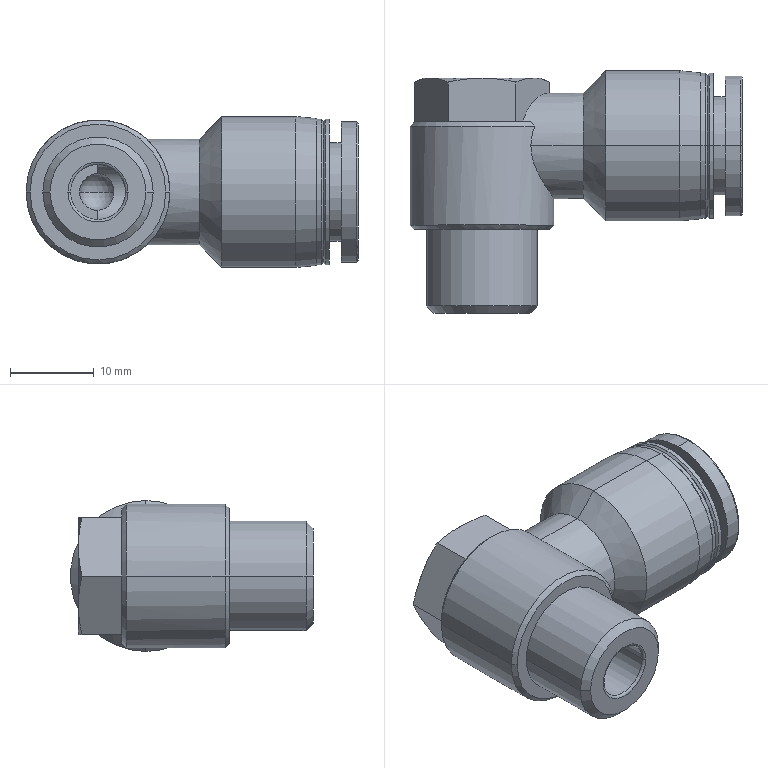Part | STEP file | PH1002 | 1 solid | 75 faces | box 39.583 x 28.95 x 18 mm | volume 7378 mm3 | cylinder 24 | plane 23 | cone 20 | torus 6 | sphere 2 | commonest cylinder face diameters 17.4 x4 4.386 x2 6.579 x2 6.667 x2 10 x2 11.8 x2